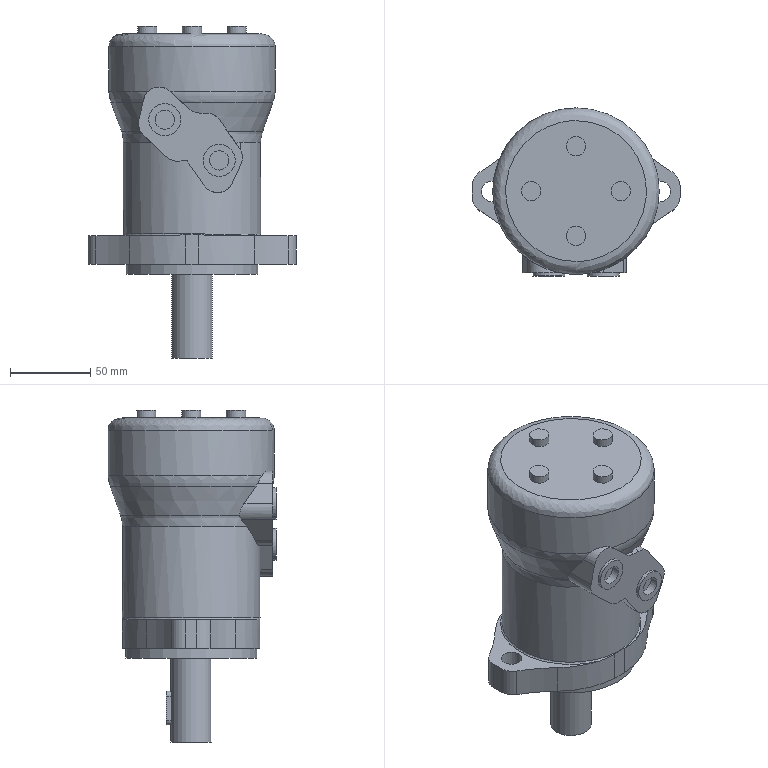Part | STEP file | MOTOR2_id434_x_t | 1 solid | 75 faces | box 130 x 105 x 207.5 mm | volume 1082578 mm3 | cylinder 39 | plane 30 | other 5 | cone 1 | commonest cylinder face diameters 20 x13 12 x6 110 x4 220 x4 6 x2 13 x2